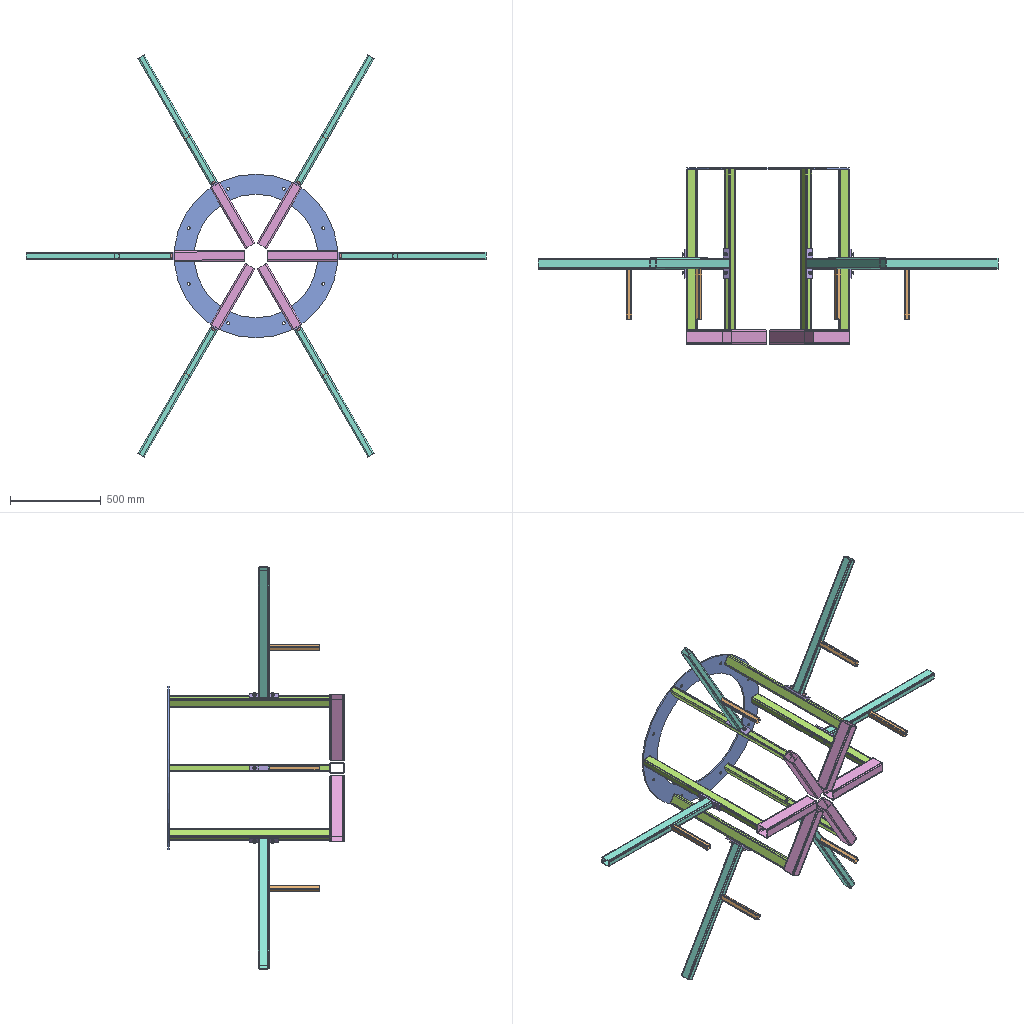Assembly | SolidWorks | 6 different items | 37 placed | box 2530 x 972 x 2211 mm
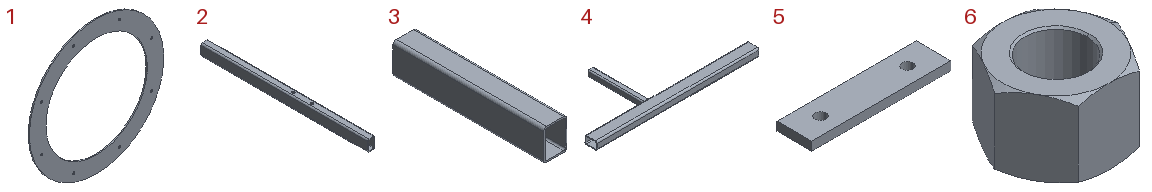Parts list (item | quantity | size | volume | features):
1 | x1 | 900 x 8 x 900 mm | 2172725 mm3 | features Extrusion 1, HoleWzd 1
2 | x6 | 40 x 884 x 60 mm | 751210 mm3 | features HoleWzd 1, WeldMemberFeat 1, WeldmentFeature 1
3 | x6 | 60 x 385 x 80 mm | 390697 mm3 | features WeldMemberFeat 1, WeldmentFeature 1
4 | x6 | 805 x 335 x 40 mm | 647000 mm3 | features WeldMemberFeat 2, WeldCornerFeat 1, WeldmentFeature 1
5 | x6 | 160 x 40 x 10 mm | 61546 mm3 | features HoleWzd 2, Extrusion 1
6 | x12 | 19.9 x 17.234 x 12.2 mm | 2145 mm3 | features Cut 2, Chamfer 1, Extrusion 1
Mates (type | each side: item.copy, entity, surface, feature):
Coincident | 1.1 face plane Boss-Extrude1 | 2.1 face plane GB/T 6728-2002 rectangular hollow section 60X40X5(1)
Coincident | 2.1 plane | assembly plane
Tangent | 1.1 face cylinder Boss-Extrude1 | 2.1 face plane GB/T 6728-2002 rectangular hollow section 60X40X5(1)
Coincident | 2.1 face plane GB/T 6728-2002 rectangular hollow section 60X40X5(1) | 3.1 face plane GB/T 6728-2002 rectangular hollow section 80X60X4(1) | 2 times
Width | 2.1 face plane GB/T 6728-2002 rectangular hollow section 60X40X5(1) | 2.1 face plane GB/T 6728-2002 rectangular hollow section 60X40X5(1) | 3.1 face plane GB/T 6728-2002 rectangular hollow section 80X60X4(1) | 3.1 face plane GB/T 6728-2002 rectangular hollow section 80X60X4(1)
Coincident | 4.1 face plane GB/T 6728-2002 rectangular hollow section 60X40X4(1) | 5.1 face plane Boss-Extrude1 | 2 times
Width | 5.1 face plane Boss-Extrude1 | 5.1 face plane Boss-Extrude1 | 4.1 face plane GB/T 6728-2002 rectangular hollow section 60X40X4(1) | 4.1 face plane GB/T 6728-2002 rectangular hollow section 60X40X4(1)
Coincident | 2.1 face plane GB/T 6728-2002 rectangular hollow section 60X40X5(1) | 5.1 face plane Boss-Extrude1
Concentric | 2.1 face cylinder Ø13.0 (13) Diameter Hole1 | 5.1 face cylinder Ø12.5 (12.5) Diameter Hole1
Parallel | 2.1 face plane GB/T 6728-2002 rectangular hollow section 60X40X5(1) | 5.1 face plane Boss-Extrude1
Concentric | 5.1 face cylinder Ø12.5 (12.5) Diameter Hole1 | 6.1 face cylinder Base-Extrude
Coincident | 5.1 face plane Boss-Extrude1 | 6.1 face plane Base-Extrude
Parallel | 5.1 face plane Boss-Extrude1 | 6.1 face plane Base-Extrude
Coincident | 6.1 face plane Base-Extrude | 6.2 face plane Base-Extrude
Parallel | 6.1 face plane Base-Extrude | 6.2 face plane Base-Extrude
Concentric | 6.2 face cylinder Base-Extrude | 5.1 face cylinder Ø12.5 (12.5) Diameter Hole1